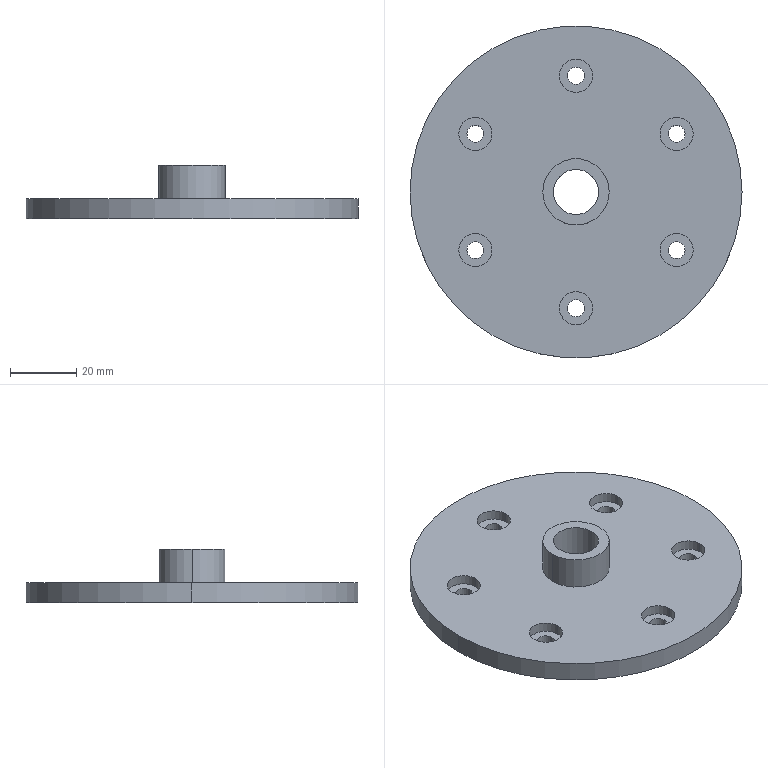NC program | NX | posted with a generic post | part box 100 x 100 x 16 mm
Whole program:
N10 G17 G21 G94 G90
(ADAPTIVE_MILLING , TOOL : D14开粗)
N12 T01 M6
N14 G53
N16 G17 G0 G90 X-66.592 Y-0.946 S4500 M3
N18 G43 Z20. H1
N20 Z-14.
N22 G94 G1 X-66.442 Y-0.942 Z-14.937 F3000.
N24 X-66.292 Y-0.937 Z-15.308
N26 X-66.142 Y-0.932 Z-15.58
N28 X-65.992 Y-0.928 Z-15.8
N30 X-65.842 Y-0.923 Z-15.984
N32 X-65.692 Y-0.918 Z-16.142
N34 X-65.542 Y-0.914 Z-16.28
N36 X-65.392 Y-0.909 Z-16.4
N38 X-65.242 Y-0.905 Z-16.505
N40 X-65.092 Y-0.9 Z-16.598
N42 X-64.942 Y-0.895 Z-16.679
N44 X-64.792 Y-0.891 Z-16.75
N46 X-64.642 Y-0.886 Z-16.81
N48 X-64.493 Y-0.881 Z-16.862
N50 X-64.343 Y-0.877 Z-16.905
N52 X-64.193 Y-0.872 Z-16.939
N54 X-64.043 Y-0.867 Z-16.966
N56 X-63.893 Y-0.863 Z-16.985
N58 X-63.743 Y-0.858 Z-16.996
N60 X-63.593 Y-0.854 Z-17.
N62 X-61.351 Y-0.784
N64 G3 X-60.09 Y0.085 R1.414
N66 X-59.182 Y3.497 R15.258
N68 G2 X-57.773 Y11.498 R186.565
N70 X-39.887 Y43.278 R59.527
N72 X-58.694 Y-4.254 R-58.855
N74 X-58.314 Y1.726 R36.055
N76 X-55.969 Y14.378 R95.392
N78 X-23.684 Y52.656 R58.108
N80 X-57.297 Y-7.015 R-57.735
N82 X-57.207 Y1.345 R41.075
N84 G3 X-57.028 Y3.729 R21.086
N86 G1 X-56.667 Y7.412
N88 X-56.069 Y11.065
N90 X-55.235 Y14.672
N92 X-54.169 Y18.216
N94 X-52.876 Y21.685
N96 X-51.361 Y25.062
N98 X-49.631 Y28.335
N100 X-47.693 Y31.488
N102 X-45.555 Y34.509
N104 X-43.225 Y37.386
N106 X-40.714 Y40.106
N108 X-38.033 Y42.657
N110 X-35.192 Y45.03
N112 X-32.203 Y47.213
N114 X-29.079 Y49.199
N116 X-25.833 Y50.978
N118 X-22.479 Y52.544
N120 X-19.03 Y53.889
N122 X-15.502 Y55.007
N124 X-11.908 Y55.896
N126 X-8.265 Y56.549
N128 X-4.587 Y56.966
N130 X-0.89 Y57.143
N132 X2.811 Y57.081
N134 X6.5 Y56.779
N136 X10.162 Y56.239
N138 X13.697 Y55.484
N140 X17.177 Y54.508
N142 X20.588 Y53.313
N144 X23.916 Y51.905
N146 X27.149 Y50.289
N148 X30.274 Y48.473
N150 X33.277 Y46.462
N152 X36.148 Y44.266
N154 X38.873 Y41.893
N156 X41.444 Y39.352
N158 X43.848 Y36.653
N160 X46.077 Y33.808
N162 X48.122 Y30.828
N164 X49.975 Y27.725
N166 X51.627 Y24.51
N168 X53.073 Y21.198
N170 X54.307 Y17.801
N172 X55.324 Y14.333
N174 X56.119 Y10.807
N176 X56.69 Y7.238
N178 X57.034 Y3.64
N180 X57.15 Y0.028
N182 X57.039 Y-3.565
N184 X56.702 Y-7.144
N186 X56.14 Y-10.695
N188 X55.357 Y-14.204
N190 X54.354 Y-17.656
N192 X53.137 Y-21.039
N194 X51.709 Y-24.338
N196 X50.076 Y-27.541
N198 X48.246 Y-30.635
N200 X46.207 Y-33.63
N202 X43.984 Y-36.49
N204 X41.583 Y-39.204
N206 X39.016 Y-41.76
N208 X36.291 Y-44.148
N210 X33.421 Y-46.359
N212 X30.416 Y-48.384
N214 X27.289 Y-50.214
N216 X24.053 Y-51.842
N218 X20.72 Y-53.262
N220 X17.303 Y-54.468
N222 X13.817 Y-55.455
N224 X10.276 Y-56.219
N226 X6.693 Y-56.757
N228 X3.083 Y-57.067
N230 X-0.539 Y-57.147
N232 X-4.159 Y-56.998
N234 X-7.762 Y-56.62
N236 X-11.334 Y-56.015
N238 X-14.861 Y-55.184
N240 X-18.327 Y-54.132
N242 X-21.72 Y-52.862
N244 X-25.026 Y-51.379
N246 X-28.231 Y-49.69
N248 X-31.323 Y-47.801
N250 X-34.289 Y-45.721
N252 X-37.117 Y-43.456
N254 X-39.796 Y-41.017
N256 X-42.315 Y-38.413
N258 X-44.664 Y-35.655
N260 X-46.833 Y-32.753
N262 X-48.815 Y-29.72
N264 X-50.531 Y-26.698
N266 X-52.06 Y-23.577
N268 X-53.397 Y-20.369
N270 X-54.536 Y-17.085
N272 X-55.474 Y-13.739
N274 X-56.207 Y-10.341
N276 X-56.731 Y-6.906
N278 X-57.046 Y-3.445
N280 X-57.15 Y0.029
N282 X-57.06 Y2.777
N284 G3 X-58.161 Y4.203 R1.414
N286 G1 X-60.404 Y4.711
N288 X-60.551 Y4.744 Z-16.996
N290 X-60.697 Y4.777 Z-16.985
N292 X-60.843 Y4.81 Z-16.966
N294 X-60.99 Y4.843 Z-16.939
N296 X-61.136 Y4.876 Z-16.905
N298 X-61.282 Y4.909 Z-16.862
N300 X-61.428 Y4.943 Z-16.81
N302 X-61.575 Y4.976 Z-16.75
N304 X-61.721 Y5.009 Z-16.679
N306 X-61.867 Y5.042 Z-16.598
N308 X-62.014 Y5.075 Z-16.505
N310 X-62.16 Y5.108 Z-16.4
N312 X-62.306 Y5.141 Z-16.28
N314 X-62.453 Y5.174 Z-16.142
N316 X-62.599 Y5.207 Z-15.984
N318 X-62.745 Y5.241 Z-15.8
N320 X-62.891 Y5.274 Z-15.58
N322 X-63.038 Y5.307 Z-15.308
N324 X-63.184 Y5.34 Z-14.937
N326 X-63.33 Y5.373 Z-14.
N328 G0 Z20.
N330 X-63.732 Y-0.929
N332 Z-6.85
N334 G1 X-63.582 Y-0.928 Z-7.787
N336 X-63.432 Y-0.926 Z-8.158
N338 X-63.282 Y-0.924 Z-8.43
N340 X-63.132 Y-0.922 Z-8.65
N342 X-62.982 Y-0.92 Z-8.834
N344 X-62.832 Y-0.919 Z-8.992
N346 X-62.682 Y-0.917 Z-9.13
N348 X-62.532 Y-0.915 Z-9.25
N350 X-62.382 Y-0.913 Z-9.355
N352 X-62.232 Y-0.911 Z-9.448
N354 X-62.082 Y-0.91 Z-9.529
N356 X-61.932 Y-0.908 Z-9.6
N358 X-61.782 Y-0.906 Z-9.66
N360 X-61.632 Y-0.904 Z-9.712
N362 X-61.482 Y-0.903 Z-9.755
N364 X-61.332 Y-0.901 Z-9.789
N366 X-61.182 Y-0.899 Z-9.816
N368 X-61.032 Y-0.897 Z-9.835
N370 X-60.882 Y-0.895 Z-9.846
N372 X-60.732 Y-0.894 Z-9.85
N374 X-58.552 Y-0.867
N376 G3 X-57.249 Y0.04 R1.414
N378 X-56.276 Y3.799 R17.53
N380 G2 X-54.643 Y12.47 R133.324
N382 X-28.763 Y48.057 R56.392
N384 X-55.836 Y-4.228 R-56.006
N386 X-55.471 Y1.629 R35.159
N388 X-53.049 Y14.262 R87.819
N390 X-21.537 Y50.477 R55.257
N392 X-54.416 Y-7.02 R-54.878
N394 X-54.308 Y1.712 R40.595
N396 X-50.589 Y18.268 R69.026
N398 X0.948 Y53.743 R53.905
N400 X-52.886 Y-9.53 R-53.748
N402 X-53.201 Y1.311 R42.329
N404 X-48.62 Y20.2 R63.036
N406 X3.228 Y52.521 R52.772
N408 X-51.336 Y-11.472 R-52.613
N410 X-52.032 Y1.586 R43.897
N412 X-46.4 Y22.355 R58.938
N414 X16.865 Y48.636 R51.548
N416 X-49.766 Y-13.105 R-51.474
N418 X-50.881 Y1.658 R44.437
N420 X-43.7 Y25.02 R56.037
N422 X46.54 Y19.175 R50.36
N424 X-48.175 Y-14.534 R-50.328
N426 X-49.711 Y1.923 R44.524
N428 X-40.923 Y27.32 R53.759
N430 X37.693 Y-31.598 R-49.194
N432 X-46.8 Y-15.069 R49.151
N434 X-48.533 Y2.231 R44.431
N436 X-38.4 Y28.886 R51.81
N438 X-23.144 Y-42.094 R-48.039
N440 X-45.62 Y-14.935 R47.654
N442 X-47.32 Y2.861 R44.313
N444 X-36.257 Y29.743 R50.176
N446 X-41.361 Y-22.072 R-46.885
N448 X-46.251 Y1.848 R42.899
N450 X-34.617 Y29.895 R48.757
N452 X-39.627 Y-22.809 R-45.726
N454 X-45.088 Y1.83 R42.158
N456 X-32.881 Y30.096 R47.296
N458 X-37.895 Y-23.441 R-44.562
N460 X-43.901 Y2.042 R41.378
N462 X-30.623 Y30.762 R45.854
N464 X-36.391 Y-23.628 R-43.393
N466 X-42.729 Y2.012 R40.499
N468 X-28.499 Y31.168 R44.468
N470 X-34.036 Y-24.977 R-42.218
N472 X-41.51 Y2.429 R39.63
N474 X-26.724 Y31.166 R43.087
N476 X-30.062 Y-27.937 R-41.04
N478 X-40.309 Y2.586 R38.739
N480 X-24.762 Y31.247 R41.743
N482 X-27.524 Y-28.824 R-39.854
N484 X-39.078 Y2.937 R37.782
N486 X-22.531 Y31.435 R40.384
N488 X-23.086 Y-31.011 R-38.661
N490 X-37.025 Y-10.286 R36.989
N492 X-34.544 Y14.995 R38.698
N494 X-9.233 Y36.303 R38.2
N496 X-29.262 Y-23.364 R-37.458
N498 X-36.65 Y3.064 R35.654
N500 X-19.093 Y30.836 R37.731
N502 X7.297 Y-35.502 R-36.254
N504 X-29.953 Y-20.344 R36.069
N506 X-35.283 Y4.158 R34.729
N508 X-17.007 Y30.649 R36.375
N510 X8.203 Y-34.052 R-35.037
N512 X-28.239 Y-20.666 R34.867
N514 X-34.069 Y4.038 R33.608
N516 X-15.414 Y30.108 R35.062
N518 X9.636 Y-32.397 R-33.811
N520 X-26.483 Y-20.949 R33.652
N522 X-32.82 Y4.082 R32.463
N524 X-13.851 Y29.498 R33.75
N526 X10.857 Y-30.7 R-32.575
N528 X-24.811 Y-21.039 R32.429
N530 X-31.586 Y3.948 R31.292
N532 X-12.131 Y28.896 R32.429
N534 X10.576 Y-29.473 R-31.326
N536 X-23.373 Y-20.786 R31.168
N538 X-30.218 Y4.529 R30.154
N540 X-10.105 Y28.329 R31.084
N542 X7.269 Y-29.158 R-30.063
N544 X-22.572 Y-19.764 R29.827
N546 X-28.75 Y5.416 R29.003
N548 X-7.681 Y27.754 R29.705
N550 X-15.591 Y-24.181 R-28.782
N552 X-27.783 Y3.675 R27.644
N554 X-7.636 Y26.43 R28.42
N556 X-5.144 Y-26.998 R-27.494
N558 X-24.924 Y-10.943 R26.592
N560 X-7.393 Y25.141 R27.126
N562 X10.925 Y-23.783 R26.191
N564 X-17.345 Y-19.531 R25.998
N566 X-24.731 Y5.497 R25.256
N568 X-3.211 Y24.655 R25.636
N570 X-10.892 Y-22.31 R-24.844
N572 X-23.574 Y4.581 R23.897
N574 X-1.594 Y23.453 R24.249
N576 X-8.613 Y-21.829 R-23.486
N578 X-22.158 Y4.623 R22.577
N580 X0.064 Y22.12 R22.826
N582 X-6.061 Y-21.23 R-22.099
N584 X-20.395 Y5.72 R21.239
N586 X1.805 Y20.617 R21.342
N588 X-4.075 Y-20.245 R-20.674
N590 X-18.738 Y6.117 R19.852
N592 X3.152 Y18.969 R19.839
N594 X-1.202 Y-19.144 R19.206
N596 X-16.071 Y8.353 R18.427
N598 X6.048 Y16.634 R18.224
N600 X0.275 Y-17.646 R17.675
N602 X-16.185 Y-5.631 R16.89
N604 X-16.768 Y-3.599 R21.233
N606 X-17.15 Y0.029 R19.984
N608 G1 X-17.032 Y2.007
N610 X-16.687 Y3.958
N612 X-16.119 Y5.857
N614 X-15.336 Y7.677
N616 X-14.348 Y9.394
N618 X-13.169 Y10.987
N620 X-11.814 Y12.432
N622 X-10.301 Y13.712
N624 X-8.651 Y14.808
N626 X-6.885 Y15.707
N628 X-5.027 Y16.397
N630 X-3.103 Y16.867
N632 X-1.136 Y17.112
N634 X0.845 Y17.129
N636 X2.815 Y16.917
N638 X4.771 Y16.473
N640 X6.662 Y15.803
N642 X8.461 Y14.917
N644 X10.145 Y13.827
N646 X11.69 Y12.548
N648 X13.075 Y11.098
N650 X14.282 Y9.495
N652 X15.293 Y7.763
N654 X16.094 Y5.924
N656 X16.676 Y4.004
N658 X17.029 Y2.03
N660 X17.15 Y0.028
N662 G2 X15.825 Y-6.61 R17.931
N664 X14.21 Y-9.602 R19.926
N666 G1 X13.047 Y-11.131
N668 X11.721 Y-12.519
N670 X10.249 Y-13.751
N672 X8.647 Y-14.81
N674 X6.938 Y-15.684
N676 X5.141 Y-16.361
N678 X3.28 Y-16.833
N680 X1.378 Y-17.095
N682 X-0.541 Y-17.141
N684 X-2.454 Y-16.973
N686 X-4.336 Y-16.593
N688 X-6.163 Y-16.004
N690 X-7.914 Y-15.215
N692 X-9.565 Y-14.235
N694 X-11.096 Y-13.077
N696 X-12.488 Y-11.755
N698 X-13.724 Y-10.285
N700 X-14.787 Y-8.687
N702 G2 X-16.217 Y-5.55 R19.305
N704 G3 X-17.646 Y-4.654 R1.414
N706 G1 X-20.012 Y-4.84
N708 X-20.162 Y-4.852 Z-9.846
N710 X-20.311 Y-4.864 Z-9.835
N712 X-20.461 Y-4.875 Z-9.816
N714 X-20.61 Y-4.887 Z-9.789
N716 X-20.76 Y-4.899 Z-9.755
N718 X-20.909 Y-4.911 Z-9.712
N720 X-21.059 Y-4.922 Z-9.66
N722 X-21.208 Y-4.934 Z-9.6
N724 X-21.358 Y-4.946 Z-9.529
N726 X-21.508 Y-4.958 Z-9.448
N728 X-21.657 Y-4.97 Z-9.355
N730 X-21.807 Y-4.981 Z-9.25
N732 X-21.956 Y-4.993 Z-9.13
N734 X-22.106 Y-5.005 Z-8.992
N736 X-22.255 Y-5.017 Z-8.834
N738 X-22.405 Y-5.029 Z-8.65
N740 X-22.554 Y-5.04 Z-8.43
N742 X-22.704 Y-5.052 Z-8.158
N744 X-22.853 Y-5.064 Z-7.787
N746 X-23.003 Y-5.076 Z-6.85
N748 G0 Z20.
(PLANAR_MILL , TOOL : D14开粗)
N750 X-20.8 Y0.
N752 Z2.
N754 G1 Z0. F1000.
N756 X-5.8
N758 G2 X0. Y5.8 R5.8
N760 X-5.8 Y0. R-5.8
N762 G1 X-20.8
N764 Z2.
N766 G0 Z20.
N768 M5
(DRILLING , TOOL : D6点钻)
N770 T03 M6
N772 G53
N774 G17 G0 G90 X-30.311 Y17.5 S2000 M3
N776 G43 Z20. H3
N778 G94 G81 G99 Z-11.5 F200. R-7.
N780 X0. Y35.
N782 X30.311 Y17.5
N784 Y-17.5
N786 X0. Y-35.
N788 X-30.311 Y-17.5
N790 G80
N792 G0 X-30.311 Y-17.5 Z20.
N794 M5
(DRILLING_COPY , TOOL : D5.1钻头)
N796 T04 M6
N798 G53
N800 G17 G0 G90 X-30.311 Y17.5 S2000 M3
N802 G43 Z20. H4
N804 G94 G83 G99 Z-19. F200. Q3. R-7.
N806 X0. Y35.
N808 X30.311 Y17.5
N810 Y-17.5
N812 X0. Y-35.
N814 X-30.311 Y-17.5
N816 G80
N818 G0 X-30.311 Y-17.5 Z20.
N820 M5
(DRILLING_COPY_COPY , TOOL : D10开粗)
N822 T05 M6
N824 G53
N826 G17 G0 G90 X-30.311 Y17.5 S1600 M3
N828 G43 Z20. H5
N830 G94 G83 G99 Z-13. F100. Q3. R-7.
N832 X0. Y35.
N834 X30.311 Y17.5
N836 Y-17.5
N838 X0. Y-35.
N840 X-30.311 Y-17.5
N842 G80
N844 G0 X-30.311 Y-17.5 Z20.
(HOLE_MILLING , TOOL : D10开粗)
N846 X0. Y0. S3500
N848 Z3.
N850 G3 X0.9 Y-0.9 R0.9 F600.
N852 X1.8 Y0. R0.9
N854 X1.8 Y0. Z2.4 I-1.8 J0.
N856 X1.8 Y0. Z1.8 I-1.8 J0.
N858 X1.8 Y0. Z1.2 I-1.8 J0.
N860 X1.8 Y0. Z0.6 I-1.8 J0.
N862 X1.8 Y0. Z0. I-1.8 J0.
N864 X1.8 Y0. Z-0.6 I-1.8 J0.
N866 X1.8 Y0. Z-1.2 I-1.8 J0.
N868 X1.8 Y0. Z-1.8 I-1.8 J0.
N870 X1.8 Y0. Z-2.4 I-1.8 J0.
N872 X1.8 Y0. Z-3. I-1.8 J0.
N874 X1.8 Y0. Z-3.6 I-1.8 J0.
N876 X1.8 Y0. Z-4.2 I-1.8 J0.
N878 X1.8 Y0. Z-4.8 I-1.8 J0.
N880 X1.8 Y0. Z-5.4 I-1.8 J0.
N882 X1.8 Y0. Z-6. I-1.8 J0.
N884 X1.8 Y0. Z-6.6 I-1.8 J0.
N886 X1.8 Y0. Z-7.2 I-1.8 J0.
N888 X1.8 Y0. Z-7.8 I-1.8 J0.
N890 X1.8 Y0. Z-8.4 I-1.8 J0.
N892 X1.8 Y0. Z-9. I-1.8 J0.
N894 X1.8 Y0. Z-9.6 I-1.8 J0.
N896 X1.8 Y0. Z-10.2 I-1.8 J0.
N898 X1.8 Y0. Z-10.8 I-1.8 J0.
N900 X1.8 Y0. Z-11.4 I-1.8 J0.
N902 X1.8 Y0. Z-12. I-1.8 J0.
N904 X1.8 Y0. Z-12.6 I-1.8 J0.
N906 X1.8 Y0. Z-13.2 I-1.8 J0.
N908 X1.8 Y0. Z-13.8 I-1.8 J0.
N910 X1.8 Y0. Z-14.4 I-1.8 J0.
N912 X1.8 Y0. Z-15. I-1.8 J0.
N914 X1.8 Y0. Z-15.6 I-1.8 J0.
N916 X1.8 Y0. Z-16.2 I-1.8 J0.
N918 X1.8 Y0. Z-16.8 I-1.8 J0.
N920 X1.8 Y0. Z-17.4 I-1.8 J0.
N922 X1.8 Y0. Z-18. I-1.8 J0.
N924 X1.8 Y0. Z-18.6 I-1.8 J0.
N926 X1.8 Y0. Z-19.2 I-1.8 J0.
N928 X1.8 Y0. Z-19.8 I-1.8 J0.
N930 X1.8 Y0. Z-20.4 I-1.8 J0.
N932 X1.8 Y0. Z-21. I-1.8 J0.
N934 X1.8 Y0. Z-21.6 I-1.8 J0.
N936 X-0.9 Y-1.559 Z-22. R-1.8
N938 X1.559 Y-0.9 R1.8
N940 X-0.9 Y-1.559 R-1.8
N942 X0.329 Y-1.229 R0.9
N944 X0. Y0. R0.9
N946 G0 Z20.
N948 M5
(PLANAR_MILL_1 , TOOL : D16精光)
N950 T02 M6
N952 G53
N954 G17 G0 G90 X-66. Y0. S3500 M3
N956 G43 Z20. H2
N958 Z-7.
N960 G94 G1 Z-10. F800.
N962 X-50.
N964 G2 X0. Y50. R50.
N966 X-50. Y0. R-50.
N968 G1 X-40.4
N970 G2 X0. Y40.4 R40.4
N972 X-40.4 Y0. R-40.4
N974 G1 X-30.8
N976 G2 X0. Y30.8 R30.8
N978 X-30.8 Y0. R-30.8
N980 G1 X-21.2
N982 G2 X0. Y21.2 R21.2
N984 X-21.2 Y0. R-21.2
N986 G1 X-18.1
N988 G2 X0. Y18.1 R18.1
N990 X-18.1 Y0. R-18.1
N992 G1 X-26.1
N994 Z-7.
N996 G0 Z20.
(PLANAR_MILL_1_COPY , TOOL : D16精光)
N998 X21.985 Y2.826
N1000 Z-7.99
N1002 G1 Z-9.99
N1004 G41 X21. Y3. D2
N1006 G3 X18. Y0. R3.
N1008 G2 X0. Y-18. R18.
N1010 X18. Y0. R-18.
N1012 G3 X21. Y-3. R3.
N1014 G40
N1016 G1 X21.985 Y-2.826
N1018 Z-7.99
N1020 G0 Z20.
(PLANAR_MILL_1_COPY_COPY , TOOL : D16精光)
N1022 X61.985 Y2.826
N1024 Z-14.99
N1026 G1 Z-16.99
N1028 G41 X61. Y3.
N1030 G3 X58. Y0. R3.
N1032 G2 X0. Y-58. R58.
N1034 X58. Y0. R-58.
N1036 G3 X61. Y-3. R3.
N1038 G40
N1040 G1 X61.985 Y-2.826
N1042 Y2.826
N1044 G41 X61. Y3.
N1046 G3 X58. Y0. R3.
N1048 G2 X0. Y-58. R58.
N1050 X58. Y0. R-58.
N1052 G3 X61. Y-3. R3.
N1054 G40
N1056 G1 X61.985 Y-2.826
N1058 Z-14.99
N1060 G0 Z20.
N1062 M5
(PLANAR_MILL_2 , TOOL : D6点钻)
N1064 T03 M6
N1066 G53
N1068 G17 G0 G90 X14.492 Y1.913 S3000 M3
N1070 G43 Z20. H3
N1072 Z0.
N1074 G94 G1 Z-2. F1000.
N1076 G41 X14. Y2. D3
N1078 G3 X12. Y0. R2.
N1080 G2 X0. Y-12. R12.
N1082 X12. Y0. R-12.
N1084 G3 X14. Y-2. R2.
N1086 G40
N1088 G1 X14.492 Y-1.913
N1090 Z0.
N1092 G0 Z20.
(PLANAR_MILL_2_COPY , TOOL : D6点钻)
N1094 X-3.587 Y0.913
N1096 Z0.
N1098 G1 Z-2.
N1100 G41 X-4.079 Y1.
N1102 X-4.2
N1104 G3 X-5.2 Y0. R1.
N1106 X0. Y-5.2 R5.2
N1108 X-5.2 Y0. R-5.2
N1110 X-4.2 Y-1. R1.
N1112 G1 X-4.079
N1114 G40
N1116 X-3.587 Y-0.913
N1118 Z0.
N1120 G0 Z20.
(PLANAR_MILL_3 , TOOL : D6点钻)
N1122 X28.311 Y18.5
N1124 Z-10.
N1126 G1 Z-12.
N1128 G3 X27.311 Y17.5 R1.
N1130 X30.311 Y14.5 R3.
N1132 X27.311 Y17.5 R-3.
N1134 X28.311 Y16.5 R1.
N1136 G1 Z-10.
N1138 G0 Z20.
N1140 X-2. Y36.
N1142 Z-10.
N1144 G1 Z-12.
N1146 G3 X-3. Y35. R1.
N1148 X0. Y32. R3.
N1150 X-3. Y35. R-3.
N1152 X-2. Y34. R1.
N1154 G1 Z-10.
N1156 G0 Z20.
N1158 X-32.311 Y18.5
N1160 Z-10.
N1162 G1 Z-12.
N1164 G3 X-33.311 Y17.5 R1.
N1166 X-30.311 Y14.5 R3.
N1168 X-33.311 Y17.5 R-3.
N1170 X-32.311 Y16.5 R1.
N1172 G1 Z-10.
N1174 G0 Z20.
N1176 Y-16.5
N1178 Z-10.
N1180 G1 Z-12.
N1182 G3 X-33.311 Y-17.5 R1.
N1184 X-30.311 Y-20.5 R3.
N1186 X-33.311 Y-17.5 R-3.
N1188 X-32.311 Y-18.5 R1.
N1190 G1 Z-10.
N1192 G0 Z20.
N1194 X-2. Y-34.
N1196 Z-10.
N1198 G1 Z-12.
N1200 G3 X-3. Y-35. R1.
N1202 X0. Y-38. R3.
N1204 X-3. Y-35. R-3.
N1206 X-2. Y-36. R1.
N1208 G1 Z-10.
N1210 G0 Z20.
N1212 X28.311 Y-16.5
N1214 Z-10.
N1216 G1 Z-12.
N1218 G3 X27.311 Y-17.5 R1.
N1220 X30.311 Y-20.5 R3.
N1222 X27.311 Y-17.5 R-3.
N1224 X28.311 Y-18.5 R1.
N1226 G1 Z-10.
N1228 G0 Z20.
(PLANAR_MILL_3_COPY , TOOL : D6点钻)
N1230 X53. Y1.
N1232 Z-10.
N1234 G1 Z-12.
N1236 G3 X52. Y0. R1.
N1238 G2 X0. Y-52. R52.
N1240 X52. Y0. R-52.
N1242 G3 X53. Y-1. R1.
N1244 G1 Z-10.
N1246 G0 Z20.
(DRILLING_COPY_1 , TOOL : D6点钻)
N1248 X-30.311 Y17.5
N1250 G81 G99 Z-15.6 F200. R-11.
N1252 G0 Z-8.
N1254 G81 X0. Y35. Z-15.6 R-11.
N1256 G0 Z-8.
N1258 G81 X30.311 Y17.5 Z-15.6 R-11.
N1260 G0 Z-8.
N1262 G81 Y-17.5 Z-15.6 R-11.
N1264 G0 Z-8.
N1266 G81 X0. Y-35. Z-15.6 R-11.
N1268 G0 Z-8.
N1270 G81 X-30.311 Y-17.5 Z-15.6 R-11.
N1272 G0 Z-8.
N1274 G80
N1276 G0 X-30.311 Y-17.5 Z20.
N1278 M5
(ADAPTIVE_MILLING_1 , TOOL : D14开粗)
N1280 T01 M6
N1282 G54
N1284 G17 G0 G90 X-66.572 Y-1.022 S4500 M3
N1286 G43 Z20. H1
N1288 Z3.15
N1290 G94 G1 X-66.422 Y-1.02 Z2.213 F3000.
N1292 X-66.272 Y-1.018 Z1.842
N1294 X-66.122 Y-1.017 Z1.57
N1296 X-65.972 Y-1.015 Z1.35
N1298 X-65.822 Y-1.013 Z1.166
N1300 X-65.672 Y-1.011 Z1.008
N1302 X-65.522 Y-1.009 Z0.87
N1304 X-65.372 Y-1.008 Z0.75
N1306 X-65.222 Y-1.006 Z0.645
N1308 X-65.072 Y-1.004 Z0.552
N1310 X-64.922 Y-1.002 Z0.471
N1312 X-64.772 Y-1. Z0.4
N1314 X-64.622 Y-0.999 Z0.34
N1316 X-64.472 Y-0.997 Z0.288
N1318 X-64.322 Y-0.995 Z0.245
N1320 X-64.172 Y-0.993 Z0.211
N1322 X-64.022 Y-0.991 Z0.184
N1324 X-63.872 Y-0.99 Z0.165
N1326 X-63.722 Y-0.988 Z0.154
N1328 X-63.572 Y-0.986 Z0.15
N1330 X-61.393 Y-0.96
N1332 G3 X-60.089 Y-0.053 R1.414
N1334 X-59.154 Y3.585 R17.128
N1336 G2 X-57.673 Y11.966 R158.261
N1338 X-34.947 Y47.361 R59.357
N1340 X-58.685 Y-4.377 R-58.856
N1342 X-58.349 Y1.356 R34.947
N1344 X-56.033 Y14.138 R95.871
N1346 X-26.829 Y51.125 R58.173
N1348 X-57.296 Y-7.014 R-57.735
N1350 X-57.163 Y1.72 R42.517
N1352 X-53.65 Y18.189 R73.711
N1354 X11. Y55.537 R56.72
N1356 X-55.826 Y-9.333 R-56.612
N1358 X-56.047 Y1.513 R44.682
N1360 X-51.481 Y20.788 R66.893
N1362 X18.711 Y52.243 R55.575
N1364 X-54.243 Y-11.643 R-55.486
N1366 X-54.91 Y1.544 R45.838
N1368 X-49.4 Y22.752 R62.785
N1370 X17.66 Y51.416 R54.447
N1372 X-52.671 Y-13.401 R-54.358
N1374 X-53.768 Y1.617 R46.514
N1376 X-47.365 Y24.34 R59.864
N1378 X16.999 Y50.444 R53.307
N1380 X-51.112 Y-14.81 R-53.225
N1382 X-52.627 Y1.659 R46.707
N1384 X-45.177 Y25.975 R57.488
N1386 X19.399 Y48.346 R52.145
N1388 X-49.584 Y-15.918 R-52.088
N1390 X-51.47 Y1.875 R46.639
N1392 X-42.648 Y27.906 R55.408
N1394 X24.205 Y44.832 R50.977
N1396 X-48.005 Y-17.025 R-50.946
N1398 X-50.3 Y2.198 R46.287
N1400 X-40.111 Y29.548 R53.533
N1402 X-9.618 Y-48.876 R-49.812
N1404 X-46.894 Y-16.7 R49.683
N1406 X-49.1 Y2.773 R45.982
N1408 X-37.352 Y31.198 R51.786
N1410 X-27.501 Y-40.137 R-48.661
N1412 X-45.867 Y-16.112 R48.092
N1414 X-47.874 Y3.504 R45.602
N1416 X-35.717 Y31.339 R50.365
N1418 X-27.987 Y-38.382 R-47.509
N1420 X-44.642 Y-16.086 R46.759
N1422 X-46.642 Y4.139 R44.954
N1424 X-33.214 Y32.342 R48.889
N1426 X-38.202 Y-26.242 R-46.352
N1428 X-45.686 Y2.132 R43.203
N1430 X-31.583 Y32.336 R47.614
N1432 X-36.905 Y-26.072 R-45.191
N1434 X-44.51 Y2.244 R42.318
N1436 X-29.401 Y32.782 R46.236
N1438 X-35.667 Y-25.796 R-44.025
N1440 X-43.332 Y2.311 R41.389
N1442 X-26.892 Y33.38 R44.88
N1444 X-34.146 Y-25.88 R-42.853
N1446 X-42.151 Y2.357 R40.435
N1448 X-25.702 Y32.825 R43.585
N1450 X-31.654 Y-27.1 R-41.677
N1452 X-40.948 Y2.564 R39.465
N1454 X-24.012 Y32.626 R42.261
N1456 X-29.319 Y-27.924 R-40.495
N1458 X-39.721 Y2.918 R38.469
N1460 X-22.147 Y32.491 R40.938
N1462 X-27.067 Y-28.491 R-39.306
N1464 X-38.512 Y3.025 R37.44
N1466 X-20.726 Y32.001 R39.655
N1468 X-21.674 Y-31.34 R-38.11
N1470 X-37.003 Y-7.573 R36.441
N1472 X-19.401 Y31.417 R38.37
N1474 X-10.82 Y-35.279 R-36.907
N1476 X-32.503 Y-17.261 R36.241
N1478 X-35.398 Y7.066 R35.817
N1480 X-15.848 Y31.998 R36.897
N1482 X-22.45 Y-27.738 R-35.692
N1484 X-34.813 Y3.464 R34.177
N1486 X-16.169 Y30.467 R35.74
N1488 X5.027 Y-34.095 R-34.475
N1490 X-27.636 Y-20.505 R34.227
N1492 X-33.303 Y5.18 R33.235
N1494 X-13.139 Y30.551 R34.359
N1496 X-4.759 Y-32.89 R-33.241
N1498 X-28.425 Y-17.003 R32.638
N1500 X-31.439 Y7.788 R32.359
N1502 X-9.97 Y30.42 R32.957
N1504 X-17.279 Y-26.919 R-31.996
N1506 X-31.08 Y3.432 R30.733
N1508 X-11.259 Y28.63 R31.792
N1510 X7.91 Y-29.699 R-30.748
N1512 X-22.831 Y-20.496 R30.514
N1514 X-29.592 Y4.705 R29.644
N1516 X-8.54 Y28.23 R30.42
N1518 X-4.945 Y-29.048 R-29.477
N1520 X-25.945 Y-13.552 R28.675
N1522 X-24.923 Y13.697 R29.019
N1524 X4.521 Y27.826 R28.69
N1526 X-16.045 Y-23.147 R-28.18
N1528 X-27.146 Y3.847 R27.121
N1530 X-5.938 Y26.248 R27.755
N1532 X-5.279 Y-26.358 R-26.893
N1534 X-24.817 Y-9.455 R25.956
N1536 X-7.187 Y24.574 R26.497
N1538 X12.538 Y-22.276 R25.586
N1540 X-16.751 Y-19.219 R25.372
N1542 X-23.985 Y5.899 R24.694
N1544 X-1.084 Y24.217 R24.943
N1546 X-9.213 Y-22.379 R-24.221
N1548 X-22.864 Y4.844 R23.316
N1550 X-0.087 Y22.874 R23.563
N1552 X-7.487 Y-21.565 R-22.85
N1554 X-21.319 Y5.278 R21.987
N1556 X1.319 Y21.432 R22.12
N1558 X-3.964 Y-21.056 R-21.448
N1560 X-19.709 Y5.704 R20.625
N1562 X2.988 Y19.805 R20.642
N1564 X-2.784 Y-19.781 R20.003
N1566 X-17.661 Y6.981 R19.213
N1568 X4.748 Y17.919 R19.099
N1570 X0.834 Y-18.465 R18.513
N1572 X-12.766 Y11.62 R17.759
N1574 X10.238 Y13.518 R17.336
N1576 X-0.96 Y-16.874 R16.926
N1578 X-2.786 Y15.176 R16.161
N1580 X14.862 Y-3.549 R15.423
N1582 X-3.898 Y-14.672 R15.133
N1584 X-4.775 Y12.883 R14.456
N1586 X13.397 Y1.597 R13.727
N1588 X-0.26 Y-13.395 R13.384
N1590 X-9.578 Y7.357 R12.642
N1592 X6.758 Y9.364 R12.029
N1594 X6.588 Y-9.304 R11.5
N1596 X-8.126 Y-7.156 R10.775
N1598 X-6.352 Y7.28 R10.274
N1600 X6.127 Y6.635 R9.524
N1602 X6.607 Y-5.685 R8.886
N1604 X-3.207 Y-7.359 R7.944
N1606 X-6.737 Y0.053 R7.025
N1608 X-3.801 Y4.033 R5.555
N1610 X-2.518 Y4.526 R37.674
N1612 G1 X-2.377 Y4.576 Z0.154
N1614 X-2.235 Y4.626 Z0.165
N1616 X-2.094 Y4.675 Z0.184
N1618 X-1.952 Y4.725 Z0.211
N1620 X-1.811 Y4.775 Z0.245
N1622 X-1.669 Y4.825 Z0.288
N1624 X-1.528 Y4.874 Z0.34
N1626 X-1.386 Y4.924 Z0.4
N1628 X-1.245 Y4.974 Z0.471
N1630 X-1.103 Y5.024 Z0.552
N1632 X-0.962 Y5.073 Z0.645
N1634 X-0.82 Y5.123 Z0.75
N1636 X-0.679 Y5.173 Z0.87
N1638 X-0.537 Y5.223 Z1.008
N1640 X-0.396 Y5.272 Z1.166
N1642 X-0.254 Y5.322 Z1.35
N1644 X-0.113 Y5.372 Z1.57
N1646 X0.029 Y5.422 Z1.842
N1648 X0.17 Y5.471 Z2.213
N1650 X0.312 Y5.521 Z3.15
N1652 G0 Z20.
N1654 M5
(FLOOR_WALL , TOOL : D16精光)
N1656 T02 M6
N1658 G54
N1660 G17 G0 G90 X0. Y-61. S3500 M3
N1662 G43 Z20. H2
N1664 Z3.
N1666 G94 G1 Z0. F1000.
N1668 Y-46.
N1670 G2 X-46. Y0. R46.
N1672 X0. Y-46. R-46.
N1674 G1 Y-34.
N1676 G2 X-34. Y0. R34.
N1678 X0. Y-34. R-34.
N1680 G1 Y-22.
N1682 G2 X-22. Y0. R22.
N1684 X0. Y-22. R-22.
N1686 G1 Y-10.
N1688 G2 X-10. Y0. R10.
N1690 X0. Y-10. R-10.
N1692 G1 Y-2.8
N1694 G2 X-2.8 Y0. R2.8
N1696 X0. Y-2.8 R-2.8
N1698 X-0.979 Y-2.623 R2.8
N1700 G1 X-2.028 Y-5.434
N1702 Z3.
N1704 G0 Z20.
N1706 M5
(PLANAR_MILL_4 , TOOL : D6点钻)
N1708 T03 M6
N1710 G54
N1712 G17 G0 G90 X-54. Y-2. S3500 M3
N1714 G43 Z20. H3
N1716 Z0.
N1718 G94 G1 Z-2. F1000.
N1720 G3 X-52. Y0. R2.
N1722 G2 X0. Y52. R52.
N1724 X-52. Y0. R-52.
N1726 G3 X-54. Y2. R2.
N1728 G1 Z0.
N1730 G0 Z20.
N1732 M5
N1734 M2